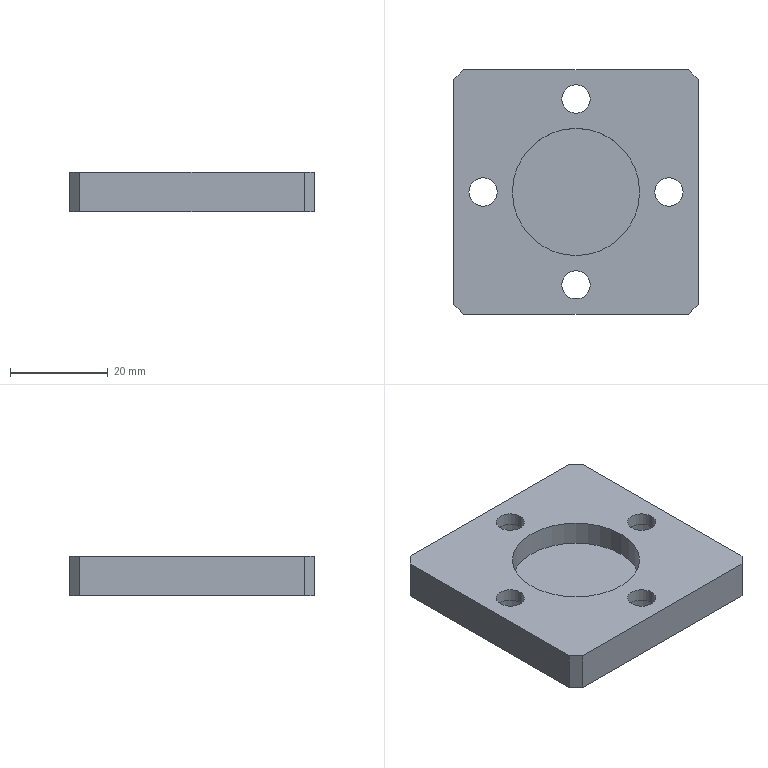Part | SolidWorks | features ICE 2, Chamfer 1, Extrusion 1, HoleWzd 1 | 1 solid | 33 faces | box 50 x 50 x 8 mm | volume 15310 mm3 | cylinder 18 | plane 15 | commonest cylinder face diameters 5.8 x8 10 x8 26 x2
STEP:
#1=CARTESIAN_POINT('',(5.,19.,1.4));
#2=VERTEX_POINT('',#1);
#3=CARTESIAN_POINT('',(-5.,19.,1.4));
#4=VERTEX_POINT('',#3);
#5=CARTESIAN_POINT('',(0.,19.,1.4));
#6=DIRECTION('',(0.,0.,-1.));
#7=DIRECTION('',(-1.,0.,0.));
#8=AXIS2_PLACEMENT_3D('',#5,#6,#7);
#9=CIRCLE('',#8,5.);
#10=EDGE_CURVE('',#2,#4,#9,.T.);
#11=ORIENTED_EDGE('',*,*,#10,.F.);
#12=CARTESIAN_POINT('',(5.,19.,-4.));
#13=VERTEX_POINT('',#12);
#14=CARTESIAN_POINT('',(5.,19.,-4.));
#15=DIRECTION('',(0.,0.,-1.));
#16=VECTOR('',#15,1000.);
#17=LINE('',#14,#16);
#18=EDGE_CURVE('',#2,#13,#17,.T.);
#19=ORIENTED_EDGE('',*,*,#18,.T.);
#20=CARTESIAN_POINT('',(-5.,19.,-4.));
#21=VERTEX_POINT('',#20);
#22=CARTESIAN_POINT('',(0.,19.,-4.));
#23=DIRECTION('',(0.,0.,-1.));
#24=DIRECTION('',(-1.,0.,0.));
#25=AXIS2_PLACEMENT_3D('',#22,#23,#24);
#26=CIRCLE('',#25,5.);
#27=EDGE_CURVE('',#13,#21,#26,.T.);
#28=ORIENTED_EDGE('',*,*,#27,.T.);
#29=CARTESIAN_POINT('',(-5.,19.,-4.));
#30=DIRECTION('',(0.,0.,-1.));
#31=VECTOR('',#30,1000.);
#32=LINE('',#29,#31);
#33=EDGE_CURVE('',#4,#21,#32,.T.);
#34=ORIENTED_EDGE('',*,*,#33,.F.);
#35=EDGE_LOOP('',(#11,#19,#28,#34));
#36=FACE_OUTER_BOUND('',#35,.T.);
#37=CARTESIAN_POINT('',(0.,19.,-4.));
#38=DIRECTION('',(0.,0.,-1.));
#39=DIRECTION('',(-1.,0.,0.));
#40=AXIS2_PLACEMENT_3D('',#37,#38,#39);
#41=CYLINDRICAL_SURFACE('',#40,5.);
#42=ADVANCED_FACE('',(#36),#41,.F.);
#43=CARTESIAN_POINT('',(2.9,19.,4.));
#44=VERTEX_POINT('',#43);
#45=CARTESIAN_POINT('',(-2.9,19.,4.));
#46=VERTEX_POINT('',#45);
#47=CARTESIAN_POINT('',(0.,19.,4.));
#48=DIRECTION('',(0.,0.,-1.));
#49=DIRECTION('',(-1.,0.,0.));
#50=AXIS2_PLACEMENT_3D('',#47,#48,#49);
#51=CIRCLE('',#50,2.9);
#52=EDGE_CURVE('',#44,#46,#51,.T.);
#53=ORIENTED_EDGE('',*,*,#52,.F.);
#54=CARTESIAN_POINT('',(2.9,19.,1.4));
#55=VERTEX_POINT('',#54);
#56=CARTESIAN_POINT('',(2.9,19.,-4.));
#57=DIRECTION('',(0.,0.,-1.));
#58=VECTOR('',#57,1000.);
#59=LINE('',#56,#58);
#60=EDGE_CURVE('',#44,#55,#59,.T.);
#61=ORIENTED_EDGE('',*,*,#60,.T.);
#62=CARTESIAN_POINT('',(-2.9,19.,1.4));
#63=VERTEX_POINT('',#62);
#64=CARTESIAN_POINT('',(0.,19.,1.4));
#65=DIRECTION('',(0.,0.,-1.));
#66=DIRECTION('',(-1.,0.,0.));
#67=AXIS2_PLACEMENT_3D('',#64,#65,#66);
#68=CIRCLE('',#67,2.9);
#69=EDGE_CURVE('',#55,#63,#68,.T.);
#70=ORIENTED_EDGE('',*,*,#69,.T.);
#71=CARTESIAN_POINT('',(-2.9,19.,-4.));
#72=DIRECTION('',(0.,0.,-1.));
#73=VECTOR('',#72,1000.);
#74=LINE('',#71,#73);
#75=EDGE_CURVE('',#46,#63,#74,.T.);
#76=ORIENTED_EDGE('',*,*,#75,.F.);
#77=EDGE_LOOP('',(#53,#61,#70,#76));
#78=FACE_OUTER_BOUND('',#77,.T.);
#79=CARTESIAN_POINT('',(0.,19.,-4.));
#80=DIRECTION('',(0.,0.,-1.));
#81=DIRECTION('',(-1.,0.,0.));
#82=AXIS2_PLACEMENT_3D('',#79,#80,#81);
#83=CYLINDRICAL_SURFACE('',#82,2.9);
#84=ADVANCED_FACE('',(#78),#83,.F.);
#85=CARTESIAN_POINT('',(24.,0.,1.4));
#86=VERTEX_POINT('',#85);
#87=CARTESIAN_POINT('',(14.,0.,1.4));
#88=VERTEX_POINT('',#87);
#89=CARTESIAN_POINT('',(19.,0.,1.4));
#90=DIRECTION('',(0.,0.,-1.));
#91=DIRECTION('',(-1.,0.,0.));
#92=AXIS2_PLACEMENT_3D('',#89,#90,#91);
#93=CIRCLE('',#92,5.);
#94=EDGE_CURVE('',#86,#88,#93,.T.);
#95=ORIENTED_EDGE('',*,*,#94,.F.);
#96=CARTESIAN_POINT('',(24.,0.,-4.));
#97=VERTEX_POINT('',#96);
#98=CARTESIAN_POINT('',(24.,0.,-4.));
#99=DIRECTION('',(0.,0.,-1.));
#100=VECTOR('',#99,1000.);
#101=LINE('',#98,#100);
#102=EDGE_CURVE('',#86,#97,#101,.T.);
#103=ORIENTED_EDGE('',*,*,#102,.T.);
#104=CARTESIAN_POINT('',(14.,0.,-4.));
#105=VERTEX_POINT('',#104);
#106=CARTESIAN_POINT('',(19.,0.,-4.));
#107=DIRECTION('',(0.,0.,-1.));
#108=DIRECTION('',(-1.,0.,0.));
#109=AXIS2_PLACEMENT_3D('',#106,#107,#108);
#110=CIRCLE('',#109,5.);
#111=EDGE_CURVE('',#97,#105,#110,.T.);
#112=ORIENTED_EDGE('',*,*,#111,.T.);
#113=CARTESIAN_POINT('',(14.,0.,-4.));
#114=DIRECTION('',(0.,0.,-1.));
#115=VECTOR('',#114,1000.);
#116=LINE('',#113,#115);
#117=EDGE_CURVE('',#88,#105,#116,.T.);
#118=ORIENTED_EDGE('',*,*,#117,.F.);
#119=EDGE_LOOP('',(#95,#103,#112,#118));
#120=FACE_OUTER_BOUND('',#119,.T.);
#121=CARTESIAN_POINT('',(19.,0.,-4.));
#122=DIRECTION('',(0.,0.,-1.));
#123=DIRECTION('',(-1.,0.,0.));
#124=AXIS2_PLACEMENT_3D('',#121,#122,#123);
#125=CYLINDRICAL_SURFACE('',#124,5.);
#126=ADVANCED_FACE('',(#120),#125,.F.);
#127=CARTESIAN_POINT('',(21.9,0.,4.));
#128=VERTEX_POINT('',#127);
#129=CARTESIAN_POINT('',(16.1,0.,4.));
#130=VERTEX_POINT('',#129);
#131=CARTESIAN_POINT('',(19.,0.,4.));
#132=DIRECTION('',(0.,0.,-1.));
#133=DIRECTION('',(-1.,0.,0.));
#134=AXIS2_PLACEMENT_3D('',#131,#132,#133);
#135=CIRCLE('',#134,2.9);
#136=EDGE_CURVE('',#128,#130,#135,.T.);
#137=ORIENTED_EDGE('',*,*,#136,.F.);
#138=CARTESIAN_POINT('',(21.9,0.,1.4));
#139=VERTEX_POINT('',#138);
#140=CARTESIAN_POINT('',(21.9,0.,-4.));
#141=DIRECTION('',(0.,0.,-1.));
#142=VECTOR('',#141,1000.);
#143=LINE('',#140,#142);
#144=EDGE_CURVE('',#128,#139,#143,.T.);
#145=ORIENTED_EDGE('',*,*,#144,.T.);
#146=CARTESIAN_POINT('',(16.1,0.,1.4));
#147=VERTEX_POINT('',#146);
#148=CARTESIAN_POINT('',(19.,0.,1.4));
#149=DIRECTION('',(0.,0.,-1.));
#150=DIRECTION('',(-1.,0.,0.));
#151=AXIS2_PLACEMENT_3D('',#148,#149,#150);
#152=CIRCLE('',#151,2.9);
#153=EDGE_CURVE('',#139,#147,#152,.T.);
#154=ORIENTED_EDGE('',*,*,#153,.T.);
#155=CARTESIAN_POINT('',(16.1,0.,-4.));
#156=DIRECTION('',(0.,0.,-1.));
#157=VECTOR('',#156,1000.);
#158=LINE('',#155,#157);
#159=EDGE_CURVE('',#130,#147,#158,.T.);
#160=ORIENTED_EDGE('',*,*,#159,.F.);
#161=EDGE_LOOP('',(#137,#145,#154,#160));
#162=FACE_OUTER_BOUND('',#161,.T.);
#163=CARTESIAN_POINT('',(19.,0.,-4.));
#164=DIRECTION('',(0.,0.,-1.));
#165=DIRECTION('',(-1.,0.,0.));
#166=AXIS2_PLACEMENT_3D('',#163,#164,#165);
#167=CYLINDRICAL_SURFACE('',#166,2.9);
#168=ADVANCED_FACE('',(#162),#167,.F.);
#169=CARTESIAN_POINT('',(5.,-19.,1.4));
#170=VERTEX_POINT('',#169);
#171=CARTESIAN_POINT('',(-5.,-19.,1.4));
#172=VERTEX_POINT('',#171);
#173=CARTESIAN_POINT('',(0.,-19.,1.4));
#174=DIRECTION('',(0.,0.,-1.));
#175=DIRECTION('',(-1.,0.,0.));
#176=AXIS2_PLACEMENT_3D('',#173,#174,#175);
#177=CIRCLE('',#176,5.);
#178=EDGE_CURVE('',#170,#172,#177,.T.);
#179=ORIENTED_EDGE('',*,*,#178,.F.);
#180=CARTESIAN_POINT('',(5.,-19.,-4.));
#181=VERTEX_POINT('',#180);
#182=CARTESIAN_POINT('',(5.,-19.,-4.));
#183=DIRECTION('',(0.,0.,-1.));
#184=VECTOR('',#183,1000.);
#185=LINE('',#182,#184);
#186=EDGE_CURVE('',#170,#181,#185,.T.);
#187=ORIENTED_EDGE('',*,*,#186,.T.);
#188=CARTESIAN_POINT('',(-5.,-19.,-4.));
#189=VERTEX_POINT('',#188);
#190=CARTESIAN_POINT('',(0.,-19.,-4.));
#191=DIRECTION('',(0.,0.,-1.));
#192=DIRECTION('',(-1.,0.,0.));
#193=AXIS2_PLACEMENT_3D('',#190,#191,#192);
#194=CIRCLE('',#193,5.);
#195=EDGE_CURVE('',#181,#189,#194,.T.);
#196=ORIENTED_EDGE('',*,*,#195,.T.);
#197=CARTESIAN_POINT('',(-5.,-19.,-4.));
#198=DIRECTION('',(0.,0.,-1.));
#199=VECTOR('',#198,1000.);
#200=LINE('',#197,#199);
#201=EDGE_CURVE('',#172,#189,#200,.T.);
#202=ORIENTED_EDGE('',*,*,#201,.F.);
#203=EDGE_LOOP('',(#179,#187,#196,#202));
#204=FACE_OUTER_BOUND('',#203,.T.);
#205=CARTESIAN_POINT('',(0.,-19.,-4.));
#206=DIRECTION('',(0.,0.,-1.));
#207=DIRECTION('',(-1.,0.,0.));
#208=AXIS2_PLACEMENT_3D('',#205,#206,#207);
#209=CYLINDRICAL_SURFACE('',#208,5.);
#210=ADVANCED_FACE('',(#204),#209,.F.);
#211=CARTESIAN_POINT('',(2.9,-19.,4.));
#212=VERTEX_POINT('',#211);
#213=CARTESIAN_POINT('',(-2.9,-19.,4.));
#214=VERTEX_POINT('',#213);
#215=CARTESIAN_POINT('',(0.,-19.,4.));
#216=DIRECTION('',(0.,0.,-1.));
#217=DIRECTION('',(-1.,0.,0.));
#218=AXIS2_PLACEMENT_3D('',#215,#216,#217);
#219=CIRCLE('',#218,2.9);
#220=EDGE_CURVE('',#212,#214,#219,.T.);
#221=ORIENTED_EDGE('',*,*,#220,.F.);
#222=CARTESIAN_POINT('',(2.9,-19.,1.4));
#223=VERTEX_POINT('',#222);
#224=CARTESIAN_POINT('',(2.9,-19.,-4.));
#225=DIRECTION('',(0.,0.,-1.));
#226=VECTOR('',#225,1000.);
#227=LINE('',#224,#226);
#228=EDGE_CURVE('',#212,#223,#227,.T.);
#229=ORIENTED_EDGE('',*,*,#228,.T.);
#230=CARTESIAN_POINT('',(-2.9,-19.,1.4));
#231=VERTEX_POINT('',#230);
#232=CARTESIAN_POINT('',(0.,-19.,1.4));
#233=DIRECTION('',(0.,0.,-1.));
#234=DIRECTION('',(-1.,0.,0.));
#235=AXIS2_PLACEMENT_3D('',#232,#233,#234);
#236=CIRCLE('',#235,2.9);
#237=EDGE_CURVE('',#223,#231,#236,.T.);
#238=ORIENTED_EDGE('',*,*,#237,.T.);
#239=CARTESIAN_POINT('',(-2.9,-19.,-4.));
#240=DIRECTION('',(0.,0.,-1.));
#241=VECTOR('',#240,1000.);
#242=LINE('',#239,#241);
#243=EDGE_CURVE('',#214,#231,#242,.T.);
#244=ORIENTED_EDGE('',*,*,#243,.F.);
#245=EDGE_LOOP('',(#221,#229,#238,#244));
#246=FACE_OUTER_BOUND('',#245,.T.);
#247=CARTESIAN_POINT('',(0.,-19.,-4.));
#248=DIRECTION('',(0.,0.,-1.));
#249=DIRECTION('',(-1.,0.,0.));
#250=AXIS2_PLACEMENT_3D('',#247,#248,#249);
#251=CYLINDRICAL_SURFACE('',#250,2.9);
#252=ADVANCED_FACE('',(#246),#251,.F.);
#253=CARTESIAN_POINT('',(-14.,0.,1.4));
#254=VERTEX_POINT('',#253);
#255=CARTESIAN_POINT('',(-24.,0.,1.4));
#256=VERTEX_POINT('',#255);
#257=CARTESIAN_POINT('',(-19.,0.,1.4));
#258=DIRECTION('',(0.,0.,-1.));
#259=DIRECTION('',(-1.,0.,0.));
#260=AXIS2_PLACEMENT_3D('',#257,#258,#259);
#261=CIRCLE('',#260,5.);
#262=EDGE_CURVE('',#254,#256,#261,.T.);
#263=ORIENTED_EDGE('',*,*,#262,.F.);
#264=CARTESIAN_POINT('',(-14.,0.,-4.));
#265=VERTEX_POINT('',#264);
#266=CARTESIAN_POINT('',(-14.,0.,-4.));
#267=DIRECTION('',(0.,0.,-1.));
#268=VECTOR('',#267,1000.);
#269=LINE('',#266,#268);
#270=EDGE_CURVE('',#254,#265,#269,.T.);
#271=ORIENTED_EDGE('',*,*,#270,.T.);
#272=CARTESIAN_POINT('',(-24.,0.,-4.));
#273=VERTEX_POINT('',#272);
#274=CARTESIAN_POINT('',(-19.,0.,-4.));
#275=DIRECTION('',(0.,0.,-1.));
#276=DIRECTION('',(-1.,0.,0.));
#277=AXIS2_PLACEMENT_3D('',#274,#275,#276);
#278=CIRCLE('',#277,5.);
#279=EDGE_CURVE('',#265,#273,#278,.T.);
#280=ORIENTED_EDGE('',*,*,#279,.T.);
#281=CARTESIAN_POINT('',(-24.,0.,-4.));
#282=DIRECTION('',(0.,0.,-1.));
#283=VECTOR('',#282,1000.);
#284=LINE('',#281,#283);
#285=EDGE_CURVE('',#256,#273,#284,.T.);
#286=ORIENTED_EDGE('',*,*,#285,.F.);
#287=EDGE_LOOP('',(#263,#271,#280,#286));
#288=FACE_OUTER_BOUND('',#287,.T.);
#289=CARTESIAN_POINT('',(-19.,0.,-4.));
#290=DIRECTION('',(0.,0.,-1.));
#291=DIRECTION('',(-1.,0.,0.));
#292=AXIS2_PLACEMENT_3D('',#289,#290,#291);
#293=CYLINDRICAL_SURFACE('',#292,5.);
#294=ADVANCED_FACE('',(#288),#293,.F.);
#295=CARTESIAN_POINT('',(-16.1,0.,4.));
#296=VERTEX_POINT('',#295);
#297=CARTESIAN_POINT('',(-21.9,0.,4.));
#298=VERTEX_POINT('',#297);
#299=CARTESIAN_POINT('',(-19.,0.,4.));
#300=DIRECTION('',(0.,0.,-1.));
#301=DIRECTION('',(-1.,0.,0.));
#302=AXIS2_PLACEMENT_3D('',#299,#300,#301);
#303=CIRCLE('',#302,2.9);
#304=EDGE_CURVE('',#296,#298,#303,.T.);
#305=ORIENTED_EDGE('',*,*,#304,.F.);
#306=CARTESIAN_POINT('',(-16.1,0.,1.4));
#307=VERTEX_POINT('',#306);
#308=CARTESIAN_POINT('',(-16.1,0.,-4.));
#309=DIRECTION('',(0.,0.,-1.));
#310=VECTOR('',#309,1000.);
#311=LINE('',#308,#310);
#312=EDGE_CURVE('',#296,#307,#311,.T.);
#313=ORIENTED_EDGE('',*,*,#312,.T.);
#314=CARTESIAN_POINT('',(-21.9,0.,1.4));
#315=VERTEX_POINT('',#314);
#316=CARTESIAN_POINT('',(-19.,0.,1.4));
#317=DIRECTION('',(0.,0.,-1.));
#318=DIRECTION('',(-1.,0.,0.));
#319=AXIS2_PLACEMENT_3D('',#316,#317,#318);
#320=CIRCLE('',#319,2.9);
#321=EDGE_CURVE('',#307,#315,#320,.T.);
#322=ORIENTED_EDGE('',*,*,#321,.T.);
#323=CARTESIAN_POINT('',(-21.9,0.,-4.));
#324=DIRECTION('',(0.,0.,-1.));
#325=VECTOR('',#324,1000.);
#326=LINE('',#323,#325);
#327=EDGE_CURVE('',#298,#315,#326,.T.);
#328=ORIENTED_EDGE('',*,*,#327,.F.);
#329=EDGE_LOOP('',(#305,#313,#322,#328));
#330=FACE_OUTER_BOUND('',#329,.T.);
#331=CARTESIAN_POINT('',(-19.,0.,-4.));
#332=DIRECTION('',(0.,0.,-1.));
#333=DIRECTION('',(-1.,0.,0.));
#334=AXIS2_PLACEMENT_3D('',#331,#332,#333);
#335=CYLINDRICAL_SURFACE('',#334,2.9);
#336=ADVANCED_FACE('',(#330),#335,.F.);
#337=CARTESIAN_POINT('',(-13.,0.,-1.));
#338=VERTEX_POINT('',#337);
#339=CARTESIAN_POINT('',(13.,0.,-1.));
#340=VERTEX_POINT('',#339);
#341=CARTESIAN_POINT('',(0.,0.,-1.));
#342=DIRECTION('',(0.,0.,1.));
#343=DIRECTION('',(1.,0.,0.));
#344=AXIS2_PLACEMENT_3D('',#341,#342,#343);
#345=CIRCLE('',#344,13.);
#346=EDGE_CURVE('',#338,#340,#345,.T.);
#347=ORIENTED_EDGE('',*,*,#346,.F.);
#348=CARTESIAN_POINT('',(-13.,0.,4.));
#349=VERTEX_POINT('',#348);
#350=CARTESIAN_POINT('',(-13.,0.,-1.));
#351=DIRECTION('',(0.,0.,1.));
#352=VECTOR('',#351,1000.);
#353=LINE('',#350,#352);
#354=EDGE_CURVE('',#338,#349,#353,.T.);
#355=ORIENTED_EDGE('',*,*,#354,.T.);
#356=CARTESIAN_POINT('',(13.,0.,4.));
#357=VERTEX_POINT('',#356);
#358=CARTESIAN_POINT('',(0.,0.,4.));
#359=DIRECTION('',(0.,0.,1.));
#360=DIRECTION('',(1.,0.,0.));
#361=AXIS2_PLACEMENT_3D('',#358,#359,#360);
#362=CIRCLE('',#361,13.);
#363=EDGE_CURVE('',#349,#357,#362,.T.);
#364=ORIENTED_EDGE('',*,*,#363,.T.);
#365=CARTESIAN_POINT('',(13.,0.,-1.));
#366=DIRECTION('',(0.,0.,1.));
#367=VECTOR('',#366,1000.);
#368=LINE('',#365,#367);
#369=EDGE_CURVE('',#340,#357,#368,.T.);
#370=ORIENTED_EDGE('',*,*,#369,.F.);
#371=EDGE_LOOP('',(#347,#355,#364,#370));
#372=FACE_OUTER_BOUND('',#371,.T.);
#373=CARTESIAN_POINT('',(0.,0.,-1.));
#374=DIRECTION('',(0.,0.,1.));
#375=DIRECTION('',(1.,0.,0.));
#376=AXIS2_PLACEMENT_3D('',#373,#374,#375);
#377=CYLINDRICAL_SURFACE('',#376,13.);
#378=ADVANCED_FACE('',(#372),#377,.F.);
#379=CARTESIAN_POINT('',(25.,-23.,4.));
#380=VERTEX_POINT('',#379);
#381=CARTESIAN_POINT('',(25.,23.,4.));
#382=VERTEX_POINT('',#381);
#383=CARTESIAN_POINT('',(25.,-25.,4.));
#384=DIRECTION('',(0.,1.,0.));
#385=VECTOR('',#384,1000.);
#386=LINE('',#383,#385);
#387=EDGE_CURVE('',#380,#382,#386,.T.);
#388=ORIENTED_EDGE('',*,*,#387,.F.);
#389=CARTESIAN_POINT('',(25.,-23.,-4.));
#390=VERTEX_POINT('',#389);
#391=CARTESIAN_POINT('',(25.,-23.,4.));
#392=DIRECTION('',(0.,0.,-1.));
#393=VECTOR('',#392,1000.);
#394=LINE('',#391,#393);
#395=EDGE_CURVE('',#380,#390,#394,.T.);
#396=ORIENTED_EDGE('',*,*,#395,.T.);
#397=CARTESIAN_POINT('',(25.,23.,-4.));
#398=VERTEX_POINT('',#397);
#399=CARTESIAN_POINT('',(25.,-25.,-4.));
#400=DIRECTION('',(0.,1.,0.));
#401=VECTOR('',#400,1000.);
#402=LINE('',#399,#401);
#403=EDGE_CURVE('',#390,#398,#402,.T.);
#404=ORIENTED_EDGE('',*,*,#403,.T.);
#405=CARTESIAN_POINT('',(25.,23.,4.));
#406=DIRECTION('',(0.,0.,1.));
#407=VECTOR('',#406,1000.);
#408=LINE('',#405,#407);
#409=EDGE_CURVE('',#398,#382,#408,.T.);
#410=ORIENTED_EDGE('',*,*,#409,.T.);
#411=EDGE_LOOP('',(#388,#396,#404,#410));
#412=FACE_OUTER_BOUND('',#411,.T.);
#413=CARTESIAN_POINT('',(25.,-25.,4.));
#414=DIRECTION('',(-1.,0.,0.));
#415=DIRECTION('',(0.,0.,1.));
#416=AXIS2_PLACEMENT_3D('',#413,#414,#415);
#417=PLANE('',#416);
#418=ADVANCED_FACE('',(#412),#417,.F.);
#419=CARTESIAN_POINT('',(23.,25.,4.));
#420=VERTEX_POINT('',#419);
#421=CARTESIAN_POINT('',(-23.,25.,4.));
#422=VERTEX_POINT('',#421);
#423=CARTESIAN_POINT('',(-25.,25.,4.));
#424=DIRECTION('',(-1.,0.,0.));
#425=VECTOR('',#424,1000.);
#426=LINE('',#423,#425);
#427=EDGE_CURVE('',#420,#422,#426,.T.);
#428=ORIENTED_EDGE('',*,*,#427,.F.);
#429=CARTESIAN_POINT('',(23.,25.,-4.));
#430=VERTEX_POINT('',#429);
#431=CARTESIAN_POINT('',(23.,25.,4.));
#432=DIRECTION('',(0.,0.,-1.));
#433=VECTOR('',#432,1000.);
#434=LINE('',#431,#433);
#435=EDGE_CURVE('',#420,#430,#434,.T.);
#436=ORIENTED_EDGE('',*,*,#435,.T.);
#437=CARTESIAN_POINT('',(-23.,25.,-4.));
#438=VERTEX_POINT('',#437);
#439=CARTESIAN_POINT('',(-25.,25.,-4.));
#440=DIRECTION('',(-1.,0.,0.));
#441=VECTOR('',#440,1000.);
#442=LINE('',#439,#441);
#443=EDGE_CURVE('',#430,#438,#442,.T.);
#444=ORIENTED_EDGE('',*,*,#443,.T.);
#445=CARTESIAN_POINT('',(-23.,25.,4.));
#446=DIRECTION('',(0.,0.,1.));
#447=VECTOR('',#446,1000.);
#448=LINE('',#445,#447);
#449=EDGE_CURVE('',#438,#422,#448,.T.);
#450=ORIENTED_EDGE('',*,*,#449,.T.);
#451=EDGE_LOOP('',(#428,#436,#444,#450));
#452=FACE_OUTER_BOUND('',#451,.T.);
#453=CARTESIAN_POINT('',(-25.,25.,4.));
#454=DIRECTION('',(0.,-1.,0.));
#455=DIRECTION('',(0.,0.,-1.));
#456=AXIS2_PLACEMENT_3D('',#453,#454,#455);
#457=PLANE('',#456);
#458=ADVANCED_FACE('',(#452),#457,.F.);
#459=CARTESIAN_POINT('',(-25.,23.,-4.));
#460=VERTEX_POINT('',#459);
#461=CARTESIAN_POINT('',(-25.,-23.,-4.));
#462=VERTEX_POINT('',#461);
#463=CARTESIAN_POINT('',(-25.,-25.,-4.));
#464=DIRECTION('',(0.,-1.,0.));
#465=VECTOR('',#464,1000.);
#466=LINE('',#463,#465);
#467=EDGE_CURVE('',#460,#462,#466,.T.);
#468=ORIENTED_EDGE('',*,*,#467,.T.);
#469=CARTESIAN_POINT('',(-25.,-23.,4.));
#470=VERTEX_POINT('',#469);
#471=CARTESIAN_POINT('',(-25.,-23.,4.));
#472=DIRECTION('',(0.,0.,1.));
#473=VECTOR('',#472,1000.);
#474=LINE('',#471,#473);
#475=EDGE_CURVE('',#462,#470,#474,.T.);
#476=ORIENTED_EDGE('',*,*,#475,.T.);
#477=CARTESIAN_POINT('',(-25.,23.,4.));
#478=VERTEX_POINT('',#477);
#479=CARTESIAN_POINT('',(-25.,-25.,4.));
#480=DIRECTION('',(0.,-1.,0.));
#481=VECTOR('',#480,1000.);
#482=LINE('',#479,#481);
#483=EDGE_CURVE('',#478,#470,#482,.T.);
#484=ORIENTED_EDGE('',*,*,#483,.F.);
#485=CARTESIAN_POINT('',(-25.,23.,4.));
#486=DIRECTION('',(0.,0.,-1.));
#487=VECTOR('',#486,1000.);
#488=LINE('',#485,#487);
#489=EDGE_CURVE('',#478,#460,#488,.T.);
#490=ORIENTED_EDGE('',*,*,#489,.T.);
#491=EDGE_LOOP('',(#468,#476,#484,#490));
#492=FACE_OUTER_BOUND('',#491,.T.);
#493=CARTESIAN_POINT('',(-25.,-25.,4.));
#494=DIRECTION('',(1.,0.,0.));
#495=DIRECTION('',(0.,0.,-1.));
#496=AXIS2_PLACEMENT_3D('',#493,#494,#495);
#497=PLANE('',#496);
#498=ADVANCED_FACE('',(#492),#497,.F.);
#499=CARTESIAN_POINT('',(-23.,-25.,4.));
#500=VERTEX_POINT('',#499);
#501=CARTESIAN_POINT('',(23.,-25.,4.));
#502=VERTEX_POINT('',#501);
#503=CARTESIAN_POINT('',(-25.,-25.,4.));
#504=DIRECTION('',(1.,0.,0.));
#505=VECTOR('',#504,1000.);
#506=LINE('',#503,#505);
#507=EDGE_CURVE('',#500,#502,#506,.T.);
#508=ORIENTED_EDGE('',*,*,#507,.F.);
#509=CARTESIAN_POINT('',(-23.,-25.,-4.));
#510=VERTEX_POINT('',#509);
#511=CARTESIAN_POINT('',(-23.,-25.,4.));
#512=DIRECTION('',(0.,0.,-1.));
#513=VECTOR('',#512,1000.);
#514=LINE('',#511,#513);
#515=EDGE_CURVE('',#500,#510,#514,.T.);
#516=ORIENTED_EDGE('',*,*,#515,.T.);
#517=CARTESIAN_POINT('',(23.,-25.,-4.));
#518=VERTEX_POINT('',#517);
#519=CARTESIAN_POINT('',(-25.,-25.,-4.));
#520=DIRECTION('',(1.,0.,0.));
#521=VECTOR('',#520,1000.);
#522=LINE('',#519,#521);
#523=EDGE_CURVE('',#510,#518,#522,.T.);
#524=ORIENTED_EDGE('',*,*,#523,.T.);
#525=CARTESIAN_POINT('',(23.,-25.,4.));
#526=DIRECTION('',(0.,0.,1.));
#527=VECTOR('',#526,1000.);
#528=LINE('',#525,#527);
#529=EDGE_CURVE('',#518,#502,#528,.T.);
#530=ORIENTED_EDGE('',*,*,#529,.T.);
#531=EDGE_LOOP('',(#508,#516,#524,#530));
#532=FACE_OUTER_BOUND('',#531,.T.);
#533=CARTESIAN_POINT('',(-25.,-25.,4.));
#534=DIRECTION('',(0.,1.,0.));
#535=DIRECTION('',(0.,0.,1.));
#536=AXIS2_PLACEMENT_3D('',#533,#534,#535);
#537=PLANE('',#536);
#538=ADVANCED_FACE('',(#532),#537,.F.);
#539=CARTESIAN_POINT('',(0.,19.,4.));
#540=DIRECTION('',(0.,0.,-1.));
#541=DIRECTION('',(-1.,0.,0.));
#542=AXIS2_PLACEMENT_3D('',#539,#540,#541);
#543=CIRCLE('',#542,2.9);
#544=EDGE_CURVE('',#46,#44,#543,.T.);
#545=ORIENTED_EDGE('',*,*,#544,.T.);
#546=ORIENTED_EDGE('',*,*,#52,.T.);
#547=EDGE_LOOP('',(#545,#546));
#548=FACE_BOUND('',#547,.T.);
#549=CARTESIAN_POINT('',(19.,0.,4.));
#550=DIRECTION('',(0.,0.,-1.));
#551=DIRECTION('',(-1.,0.,0.));
#552=AXIS2_PLACEMENT_3D('',#549,#550,#551);
#553=CIRCLE('',#552,2.9);
#554=EDGE_CURVE('',#130,#128,#553,.T.);
#555=ORIENTED_EDGE('',*,*,#554,.T.);
#556=ORIENTED_EDGE('',*,*,#136,.T.);
#557=EDGE_LOOP('',(#555,#556));
#558=FACE_BOUND('',#557,.T.);
#559=CARTESIAN_POINT('',(0.,-19.,4.));
#560=DIRECTION('',(0.,0.,-1.));
#561=DIRECTION('',(-1.,0.,0.));
#562=AXIS2_PLACEMENT_3D('',#559,#560,#561);
#563=CIRCLE('',#562,2.9);
#564=EDGE_CURVE('',#214,#212,#563,.T.);
#565=ORIENTED_EDGE('',*,*,#564,.T.);
#566=ORIENTED_EDGE('',*,*,#220,.T.);
#567=EDGE_LOOP('',(#565,#566));
#568=FACE_BOUND('',#567,.T.);
#569=CARTESIAN_POINT('',(-19.,0.,4.));
#570=DIRECTION('',(0.,0.,-1.));
#571=DIRECTION('',(-1.,0.,0.));
#572=AXIS2_PLACEMENT_3D('',#569,#570,#571);
#573=CIRCLE('',#572,2.9);
#574=EDGE_CURVE('',#298,#296,#573,.T.);
#575=ORIENTED_EDGE('',*,*,#574,.T.);
#576=ORIENTED_EDGE('',*,*,#304,.T.);
#577=EDGE_LOOP('',(#575,#576));
#578=FACE_BOUND('',#577,.T.);
#579=CARTESIAN_POINT('',(0.,0.,4.));
#580=DIRECTION('',(0.,0.,1.));
#581=DIRECTION('',(1.,0.,0.));
#582=AXIS2_PLACEMENT_3D('',#579,#580,#581);
#583=CIRCLE('',#582,13.);
#584=EDGE_CURVE('',#357,#349,#583,.T.);
#585=ORIENTED_EDGE('',*,*,#584,.F.);
#586=ORIENTED_EDGE('',*,*,#363,.F.);
#587=EDGE_LOOP('',(#585,#586));
#588=FACE_BOUND('',#587,.T.);
#589=ORIENTED_EDGE('',*,*,#483,.T.);
#590=CARTESIAN_POINT('',(-23.,-25.,4.));
#591=DIRECTION('',(0.7071,-0.7071,0.));
#592=VECTOR('',#591,1000.);
#593=LINE('',#590,#592);
#594=EDGE_CURVE('',#470,#500,#593,.T.);
#595=ORIENTED_EDGE('',*,*,#594,.T.);
#596=ORIENTED_EDGE('',*,*,#507,.T.);
#597=CARTESIAN_POINT('',(25.,-23.,4.));
#598=DIRECTION('',(0.7071,0.7071,0.));
#599=VECTOR('',#598,1000.);
#600=LINE('',#597,#599);
#601=EDGE_CURVE('',#502,#380,#600,.T.);
#602=ORIENTED_EDGE('',*,*,#601,.T.);
#603=ORIENTED_EDGE('',*,*,#387,.T.);
#604=CARTESIAN_POINT('',(23.,25.,4.));
#605=DIRECTION('',(-0.7071,0.7071,0.));
#606=VECTOR('',#605,1000.);
#607=LINE('',#604,#606);
#608=EDGE_CURVE('',#382,#420,#607,.T.);
#609=ORIENTED_EDGE('',*,*,#608,.T.);
#610=ORIENTED_EDGE('',*,*,#427,.T.);
#611=CARTESIAN_POINT('',(-25.,23.,4.));
#612=DIRECTION('',(-0.7071,-0.7071,0.));
#613=VECTOR('',#612,1000.);
#614=LINE('',#611,#613);
#615=EDGE_CURVE('',#422,#478,#614,.T.);
#616=ORIENTED_EDGE('',*,*,#615,.T.);
#617=EDGE_LOOP('',(#589,#595,#596,#602,#603,#609,#610,#616));
#618=FACE_OUTER_BOUND('',#617,.T.);
#619=CARTESIAN_POINT('',(0.,0.,4.));
#620=DIRECTION('',(0.,0.,-1.));
#621=DIRECTION('',(-1.,0.,0.));
#622=AXIS2_PLACEMENT_3D('',#619,#620,#621);
#623=PLANE('',#622);
#624=ADVANCED_FACE('',(#548,#558,#568,#578,#588,#618),#623,.F.);
#625=CARTESIAN_POINT('',(0.,19.,-4.));
#626=DIRECTION('',(0.,0.,-1.));
#627=DIRECTION('',(-1.,0.,0.));
#628=AXIS2_PLACEMENT_3D('',#625,#626,#627);
#629=CIRCLE('',#628,5.);
#630=EDGE_CURVE('',#21,#13,#629,.T.);
#631=ORIENTED_EDGE('',*,*,#630,.F.);
#632=ORIENTED_EDGE('',*,*,#27,.F.);
#633=EDGE_LOOP('',(#631,#632));
#634=FACE_BOUND('',#633,.T.);
#635=CARTESIAN_POINT('',(19.,0.,-4.));
#636=DIRECTION('',(0.,0.,-1.));
#637=DIRECTION('',(-1.,0.,0.));
#638=AXIS2_PLACEMENT_3D('',#635,#636,#637);
#639=CIRCLE('',#638,5.);
#640=EDGE_CURVE('',#105,#97,#639,.T.);
#641=ORIENTED_EDGE('',*,*,#640,.F.);
#642=ORIENTED_EDGE('',*,*,#111,.F.);
#643=EDGE_LOOP('',(#641,#642));
#644=FACE_BOUND('',#643,.T.);
#645=CARTESIAN_POINT('',(0.,-19.,-4.));
#646=DIRECTION('',(0.,0.,-1.));
#647=DIRECTION('',(-1.,0.,0.));
#648=AXIS2_PLACEMENT_3D('',#645,#646,#647);
#649=CIRCLE('',#648,5.);
#650=EDGE_CURVE('',#189,#181,#649,.T.);
#651=ORIENTED_EDGE('',*,*,#650,.F.);
#652=ORIENTED_EDGE('',*,*,#195,.F.);
#653=EDGE_LOOP('',(#651,#652));
#654=FACE_BOUND('',#653,.T.);
#655=CARTESIAN_POINT('',(-19.,0.,-4.));
#656=DIRECTION('',(0.,0.,-1.));
#657=DIRECTION('',(-1.,0.,0.));
#658=AXIS2_PLACEMENT_3D('',#655,#656,#657);
#659=CIRCLE('',#658,5.);
#660=EDGE_CURVE('',#273,#265,#659,.T.);
#661=ORIENTED_EDGE('',*,*,#660,.F.);
#662=ORIENTED_EDGE('',*,*,#279,.F.);
#663=EDGE_LOOP('',(#661,#662));
#664=FACE_BOUND('',#663,.T.);
#665=ORIENTED_EDGE('',*,*,#523,.F.);
#666=CARTESIAN_POINT('',(-24.,-24.,-4.));
#667=DIRECTION('',(-0.7071,0.7071,0.));
#668=VECTOR('',#667,1000.);
#669=LINE('',#666,#668);
#670=EDGE_CURVE('',#510,#462,#669,.T.);
#671=ORIENTED_EDGE('',*,*,#670,.T.);
#672=ORIENTED_EDGE('',*,*,#467,.F.);
#673=CARTESIAN_POINT('',(-24.,24.,-4.));
#674=DIRECTION('',(0.7071,0.7071,0.));
#675=VECTOR('',#674,1000.);
#676=LINE('',#673,#675);
#677=EDGE_CURVE('',#460,#438,#676,.T.);
#678=ORIENTED_EDGE('',*,*,#677,.T.);
#679=ORIENTED_EDGE('',*,*,#443,.F.);
#680=CARTESIAN_POINT('',(24.,24.,-4.));
#681=DIRECTION('',(0.7071,-0.7071,0.));
#682=VECTOR('',#681,1000.);
#683=LINE('',#680,#682);
#684=EDGE_CURVE('',#430,#398,#683,.T.);
#685=ORIENTED_EDGE('',*,*,#684,.T.);
#686=ORIENTED_EDGE('',*,*,#403,.F.);
#687=CARTESIAN_POINT('',(24.,-24.,-4.));
#688=DIRECTION('',(-0.7071,-0.7071,0.));
#689=VECTOR('',#688,1000.);
#690=LINE('',#687,#689);
#691=EDGE_CURVE('',#390,#518,#690,.T.);
#692=ORIENTED_EDGE('',*,*,#691,.T.);
#693=EDGE_LOOP('',(#665,#671,#672,#678,#679,#685,#686,#692));
#694=FACE_OUTER_BOUND('',#693,.T.);
#695=CARTESIAN_POINT('',(0.,0.,-4.));
#696=DIRECTION('',(0.,0.,-1.));
#697=DIRECTION('',(-1.,0.,0.));
#698=AXIS2_PLACEMENT_3D('',#695,#696,#697);
#699=PLANE('',#698);
#700=ADVANCED_FACE('',(#634,#644,#654,#664,#694),#699,.T.);
#701=ORIENTED_EDGE('',*,*,#354,.F.);
#702=CARTESIAN_POINT('',(0.,0.,-1.));
#703=DIRECTION('',(0.,0.,1.));
#704=DIRECTION('',(1.,0.,0.));
#705=AXIS2_PLACEMENT_3D('',#702,#703,#704);
#706=CIRCLE('',#705,13.);
#707=EDGE_CURVE('',#340,#338,#706,.T.);
#708=ORIENTED_EDGE('',*,*,#707,.F.);
#709=ORIENTED_EDGE('',*,*,#369,.T.);
#710=ORIENTED_EDGE('',*,*,#584,.T.);
#711=EDGE_LOOP('',(#701,#708,#709,#710));
#712=FACE_OUTER_BOUND('',#711,.T.);
#713=CARTESIAN_POINT('',(0.,0.,-1.));
#714=DIRECTION('',(0.,0.,1.));
#715=DIRECTION('',(1.,0.,0.));
#716=AXIS2_PLACEMENT_3D('',#713,#714,#715);
#717=CYLINDRICAL_SURFACE('',#716,13.);
#718=ADVANCED_FACE('',(#712),#717,.F.);
#719=ORIENTED_EDGE('',*,*,#707,.T.);
#720=ORIENTED_EDGE('',*,*,#346,.T.);
#721=EDGE_LOOP('',(#719,#720));
#722=FACE_OUTER_BOUND('',#721,.T.);
#723=CARTESIAN_POINT('',(0.,0.,-1.));
#724=DIRECTION('',(0.,0.,1.));
#725=DIRECTION('',(1.,0.,0.));
#726=AXIS2_PLACEMENT_3D('',#723,#724,#725);
#727=PLANE('',#726);
#728=ADVANCED_FACE('',(#722),#727,.T.);
#729=ORIENTED_EDGE('',*,*,#312,.F.);
#730=ORIENTED_EDGE('',*,*,#574,.F.);
#731=ORIENTED_EDGE('',*,*,#327,.T.);
#732=CARTESIAN_POINT('',(-19.,0.,1.4));
#733=DIRECTION('',(0.,0.,-1.));
#734=DIRECTION('',(-1.,0.,0.));
#735=AXIS2_PLACEMENT_3D('',#732,#733,#734);
#736=CIRCLE('',#735,2.9);
#737=EDGE_CURVE('',#315,#307,#736,.T.);
#738=ORIENTED_EDGE('',*,*,#737,.T.);
#739=EDGE_LOOP('',(#729,#730,#731,#738));
#740=FACE_OUTER_BOUND('',#739,.T.);
#741=CARTESIAN_POINT('',(-19.,0.,-4.));
#742=DIRECTION('',(0.,0.,-1.));
#743=DIRECTION('',(-1.,0.,0.));
#744=AXIS2_PLACEMENT_3D('',#741,#742,#743);
#745=CYLINDRICAL_SURFACE('',#744,2.9);
#746=ADVANCED_FACE('',(#740),#745,.F.);
#747=ORIENTED_EDGE('',*,*,#737,.F.);
#748=ORIENTED_EDGE('',*,*,#321,.F.);
#749=EDGE_LOOP('',(#747,#748));
#750=FACE_BOUND('',#749,.T.);
#751=CARTESIAN_POINT('',(-19.,0.,1.4));
#752=DIRECTION('',(0.,0.,-1.));
#753=DIRECTION('',(-1.,0.,0.));
#754=AXIS2_PLACEMENT_3D('',#751,#752,#753);
#755=CIRCLE('',#754,5.);
#756=EDGE_CURVE('',#256,#254,#755,.T.);
#757=ORIENTED_EDGE('',*,*,#756,.T.);
#758=ORIENTED_EDGE('',*,*,#262,.T.);
#759=EDGE_LOOP('',(#757,#758));
#760=FACE_OUTER_BOUND('',#759,.T.);
#761=CARTESIAN_POINT('',(-16.1,0.,1.4));
#762=DIRECTION('',(0.,0.,1.));
#763=DIRECTION('',(1.,0.,0.));
#764=AXIS2_PLACEMENT_3D('',#761,#762,#763);
#765=PLANE('',#764);
#766=ADVANCED_FACE('',(#750,#760),#765,.F.);
#767=ORIENTED_EDGE('',*,*,#270,.F.);
#768=ORIENTED_EDGE('',*,*,#756,.F.);
#769=ORIENTED_EDGE('',*,*,#285,.T.);
#770=ORIENTED_EDGE('',*,*,#660,.T.);
#771=EDGE_LOOP('',(#767,#768,#769,#770));
#772=FACE_OUTER_BOUND('',#771,.T.);
#773=CARTESIAN_POINT('',(-19.,0.,-4.));
#774=DIRECTION('',(0.,0.,-1.));
#775=DIRECTION('',(-1.,0.,0.));
#776=AXIS2_PLACEMENT_3D('',#773,#774,#775);
#777=CYLINDRICAL_SURFACE('',#776,5.);
#778=ADVANCED_FACE('',(#772),#777,.F.);
#779=ORIENTED_EDGE('',*,*,#228,.F.);
#780=ORIENTED_EDGE('',*,*,#564,.F.);
#781=ORIENTED_EDGE('',*,*,#243,.T.);
#782=CARTESIAN_POINT('',(0.,-19.,1.4));
#783=DIRECTION('',(0.,0.,-1.));
#784=DIRECTION('',(-1.,0.,0.));
#785=AXIS2_PLACEMENT_3D('',#782,#783,#784);
#786=CIRCLE('',#785,2.9);
#787=EDGE_CURVE('',#231,#223,#786,.T.);
#788=ORIENTED_EDGE('',*,*,#787,.T.);
#789=EDGE_LOOP('',(#779,#780,#781,#788));
#790=FACE_OUTER_BOUND('',#789,.T.);
#791=CARTESIAN_POINT('',(0.,-19.,-4.));
#792=DIRECTION('',(0.,0.,-1.));
#793=DIRECTION('',(-1.,0.,0.));
#794=AXIS2_PLACEMENT_3D('',#791,#792,#793);
#795=CYLINDRICAL_SURFACE('',#794,2.9);
#796=ADVANCED_FACE('',(#790),#795,.F.);
#797=ORIENTED_EDGE('',*,*,#787,.F.);
#798=ORIENTED_EDGE('',*,*,#237,.F.);
#799=EDGE_LOOP('',(#797,#798));
#800=FACE_BOUND('',#799,.T.);
#801=CARTESIAN_POINT('',(0.,-19.,1.4));
#802=DIRECTION('',(0.,0.,-1.));
#803=DIRECTION('',(-1.,0.,0.));
#804=AXIS2_PLACEMENT_3D('',#801,#802,#803);
#805=CIRCLE('',#804,5.);
#806=EDGE_CURVE('',#172,#170,#805,.T.);
#807=ORIENTED_EDGE('',*,*,#806,.T.);
#808=ORIENTED_EDGE('',*,*,#178,.T.);
#809=EDGE_LOOP('',(#807,#808));
#810=FACE_OUTER_BOUND('',#809,.T.);
#811=CARTESIAN_POINT('',(2.9,-19.,1.4));
#812=DIRECTION('',(0.,0.,1.));
#813=DIRECTION('',(1.,0.,0.));
#814=AXIS2_PLACEMENT_3D('',#811,#812,#813);
#815=PLANE('',#814);
#816=ADVANCED_FACE('',(#800,#810),#815,.F.);
#817=ORIENTED_EDGE('',*,*,#186,.F.);
#818=ORIENTED_EDGE('',*,*,#806,.F.);
#819=ORIENTED_EDGE('',*,*,#201,.T.);
#820=ORIENTED_EDGE('',*,*,#650,.T.);
#821=EDGE_LOOP('',(#817,#818,#819,#820));
#822=FACE_OUTER_BOUND('',#821,.T.);
#823=CARTESIAN_POINT('',(0.,-19.,-4.));
#824=DIRECTION('',(0.,0.,-1.));
#825=DIRECTION('',(-1.,0.,0.));
#826=AXIS2_PLACEMENT_3D('',#823,#824,#825);
#827=CYLINDRICAL_SURFACE('',#826,5.);
#828=ADVANCED_FACE('',(#822),#827,.F.);
#829=ORIENTED_EDGE('',*,*,#144,.F.);
#830=ORIENTED_EDGE('',*,*,#554,.F.);
#831=ORIENTED_EDGE('',*,*,#159,.T.);
#832=CARTESIAN_POINT('',(19.,0.,1.4));
#833=DIRECTION('',(0.,0.,-1.));
#834=DIRECTION('',(-1.,0.,0.));
#835=AXIS2_PLACEMENT_3D('',#832,#833,#834);
#836=CIRCLE('',#835,2.9);
#837=EDGE_CURVE('',#147,#139,#836,.T.);
#838=ORIENTED_EDGE('',*,*,#837,.T.);
#839=EDGE_LOOP('',(#829,#830,#831,#838));
#840=FACE_OUTER_BOUND('',#839,.T.);
#841=CARTESIAN_POINT('',(19.,0.,-4.));
#842=DIRECTION('',(0.,0.,-1.));
#843=DIRECTION('',(-1.,0.,0.));
#844=AXIS2_PLACEMENT_3D('',#841,#842,#843);
#845=CYLINDRICAL_SURFACE('',#844,2.9);
#846=ADVANCED_FACE('',(#840),#845,.F.);
#847=ORIENTED_EDGE('',*,*,#837,.F.);
#848=ORIENTED_EDGE('',*,*,#153,.F.);
#849=EDGE_LOOP('',(#847,#848));
#850=FACE_BOUND('',#849,.T.);
#851=CARTESIAN_POINT('',(19.,0.,1.4));
#852=DIRECTION('',(0.,0.,-1.));
#853=DIRECTION('',(-1.,0.,0.));
#854=AXIS2_PLACEMENT_3D('',#851,#852,#853);
#855=CIRCLE('',#854,5.);
#856=EDGE_CURVE('',#88,#86,#855,.T.);
#857=ORIENTED_EDGE('',*,*,#856,.T.);
#858=ORIENTED_EDGE('',*,*,#94,.T.);
#859=EDGE_LOOP('',(#857,#858));
#860=FACE_OUTER_BOUND('',#859,.T.);
#861=CARTESIAN_POINT('',(21.9,0.,1.4));
#862=DIRECTION('',(0.,0.,1.));
#863=DIRECTION('',(1.,0.,0.));
#864=AXIS2_PLACEMENT_3D('',#861,#862,#863);
#865=PLANE('',#864);
#866=ADVANCED_FACE('',(#850,#860),#865,.F.);
#867=ORIENTED_EDGE('',*,*,#102,.F.);
#868=ORIENTED_EDGE('',*,*,#856,.F.);
#869=ORIENTED_EDGE('',*,*,#117,.T.);
#870=ORIENTED_EDGE('',*,*,#640,.T.);
#871=EDGE_LOOP('',(#867,#868,#869,#870));
#872=FACE_OUTER_BOUND('',#871,.T.);
#873=CARTESIAN_POINT('',(19.,0.,-4.));
#874=DIRECTION('',(0.,0.,-1.));
#875=DIRECTION('',(-1.,0.,0.));
#876=AXIS2_PLACEMENT_3D('',#873,#874,#875);
#877=CYLINDRICAL_SURFACE('',#876,5.);
#878=ADVANCED_FACE('',(#872),#877,.F.);
#879=ORIENTED_EDGE('',*,*,#60,.F.);
#880=ORIENTED_EDGE('',*,*,#544,.F.);
#881=ORIENTED_EDGE('',*,*,#75,.T.);
#882=CARTESIAN_POINT('',(0.,19.,1.4));
#883=DIRECTION('',(0.,0.,-1.));
#884=DIRECTION('',(-1.,0.,0.));
#885=AXIS2_PLACEMENT_3D('',#882,#883,#884);
#886=CIRCLE('',#885,2.9);
#887=EDGE_CURVE('',#63,#55,#886,.T.);
#888=ORIENTED_EDGE('',*,*,#887,.T.);
#889=EDGE_LOOP('',(#879,#880,#881,#888));
#890=FACE_OUTER_BOUND('',#889,.T.);
#891=CARTESIAN_POINT('',(0.,19.,-4.));
#892=DIRECTION('',(0.,0.,-1.));
#893=DIRECTION('',(-1.,0.,0.));
#894=AXIS2_PLACEMENT_3D('',#891,#892,#893);
#895=CYLINDRICAL_SURFACE('',#894,2.9);
#896=ADVANCED_FACE('',(#890),#895,.F.);
#897=ORIENTED_EDGE('',*,*,#887,.F.);
#898=ORIENTED_EDGE('',*,*,#69,.F.);
#899=EDGE_LOOP('',(#897,#898));
#900=FACE_BOUND('',#899,.T.);
#901=CARTESIAN_POINT('',(0.,19.,1.4));
#902=DIRECTION('',(0.,0.,-1.));
#903=DIRECTION('',(-1.,0.,0.));
#904=AXIS2_PLACEMENT_3D('',#901,#902,#903);
#905=CIRCLE('',#904,5.);
#906=EDGE_CURVE('',#4,#2,#905,.T.);
#907=ORIENTED_EDGE('',*,*,#906,.T.);
#908=ORIENTED_EDGE('',*,*,#10,.T.);
#909=EDGE_LOOP('',(#907,#908));
#910=FACE_OUTER_BOUND('',#909,.T.);
#911=CARTESIAN_POINT('',(2.9,19.,1.4));
#912=DIRECTION('',(0.,0.,1.));
#913=DIRECTION('',(1.,0.,0.));
#914=AXIS2_PLACEMENT_3D('',#911,#912,#913);
#915=PLANE('',#914);
#916=ADVANCED_FACE('',(#900,#910),#915,.F.);
#917=ORIENTED_EDGE('',*,*,#18,.F.);
#918=ORIENTED_EDGE('',*,*,#906,.F.);
#919=ORIENTED_EDGE('',*,*,#33,.T.);
#920=ORIENTED_EDGE('',*,*,#630,.T.);
#921=EDGE_LOOP('',(#917,#918,#919,#920));
#922=FACE_OUTER_BOUND('',#921,.T.);
#923=CARTESIAN_POINT('',(0.,19.,-4.));
#924=DIRECTION('',(0.,0.,-1.));
#925=DIRECTION('',(-1.,0.,0.));
#926=AXIS2_PLACEMENT_3D('',#923,#924,#925);
#927=CYLINDRICAL_SURFACE('',#926,5.);
#928=ADVANCED_FACE('',(#922),#927,.F.);
#929=ORIENTED_EDGE('',*,*,#594,.F.);
#930=ORIENTED_EDGE('',*,*,#475,.F.);
#931=ORIENTED_EDGE('',*,*,#670,.F.);
#932=ORIENTED_EDGE('',*,*,#515,.F.);
#933=EDGE_LOOP('',(#929,#930,#931,#932));
#934=FACE_OUTER_BOUND('',#933,.T.);
#935=CARTESIAN_POINT('',(-23.,-25.,4.));
#936=DIRECTION('',(0.7071,0.7071,0.));
#937=DIRECTION('',(0.,0.,-1.));
#938=AXIS2_PLACEMENT_3D('',#935,#936,#937);
#939=PLANE('',#938);
#940=ADVANCED_FACE('',(#934),#939,.F.);
#941=ORIENTED_EDGE('',*,*,#601,.F.);
#942=ORIENTED_EDGE('',*,*,#529,.F.);
#943=ORIENTED_EDGE('',*,*,#691,.F.);
#944=ORIENTED_EDGE('',*,*,#395,.F.);
#945=EDGE_LOOP('',(#941,#942,#943,#944));
#946=FACE_OUTER_BOUND('',#945,.T.);
#947=CARTESIAN_POINT('',(25.,-23.,4.));
#948=DIRECTION('',(-0.7071,0.7071,0.));
#949=DIRECTION('',(0.,0.,-1.));
#950=AXIS2_PLACEMENT_3D('',#947,#948,#949);
#951=PLANE('',#950);
#952=ADVANCED_FACE('',(#946),#951,.F.);
#953=ORIENTED_EDGE('',*,*,#608,.F.);
#954=ORIENTED_EDGE('',*,*,#409,.F.);
#955=ORIENTED_EDGE('',*,*,#684,.F.);
#956=ORIENTED_EDGE('',*,*,#435,.F.);
#957=EDGE_LOOP('',(#953,#954,#955,#956));
#958=FACE_OUTER_BOUND('',#957,.T.);
#959=CARTESIAN_POINT('',(23.,25.,4.));
#960=DIRECTION('',(-0.7071,-0.7071,0.));
#961=DIRECTION('',(0.,0.,-1.));
#962=AXIS2_PLACEMENT_3D('',#959,#960,#961);
#963=PLANE('',#962);
#964=ADVANCED_FACE('',(#958),#963,.F.);
#965=ORIENTED_EDGE('',*,*,#615,.F.);
#966=ORIENTED_EDGE('',*,*,#449,.F.);
#967=ORIENTED_EDGE('',*,*,#677,.F.);
#968=ORIENTED_EDGE('',*,*,#489,.F.);
#969=EDGE_LOOP('',(#965,#966,#967,#968));
#970=FACE_OUTER_BOUND('',#969,.T.);
#971=CARTESIAN_POINT('',(-25.,23.,4.));
#972=DIRECTION('',(0.7071,-0.7071,0.));
#973=DIRECTION('',(0.,0.,-1.));
#974=AXIS2_PLACEMENT_3D('',#971,#972,#973);
#975=PLANE('',#974);
#976=ADVANCED_FACE('',(#970),#975,.F.);
#977=CLOSED_SHELL('',(#42,#84,#126,#168,#210,#252,#294,#336,#378,#418,#458,#498,#538,#624,#700,#718,#728,#746,#766,#778,#796,#816,#828,#846,#866,#878,#896,#916,#928,#940,#952,#964,#976));
#978=MANIFOLD_SOLID_BREP('',#977);
#979=CARTESIAN_POINT('',(0.,0.,0.));
#980=DIRECTION('',(0.,0.,1.));
#981=DIRECTION('',(1.,0.,0.));
#982=AXIS2_PLACEMENT_3D('',#979,#980,#981);
#983=(LENGTH_UNIT()NAMED_UNIT(*)SI_UNIT(.MILLI.,.METRE.));
#984=UNCERTAINTY_MEASURE_WITH_UNIT(LENGTH_MEASURE(0.00001),#983,'','');
#985=(NAMED_UNIT(*)PLANE_ANGLE_UNIT()SI_UNIT($,.RADIAN.));
#986=(NAMED_UNIT(*)SI_UNIT($,.STERADIAN.)SOLID_ANGLE_UNIT());
#987=(GEOMETRIC_REPRESENTATION_CONTEXT(3)GLOBAL_UNCERTAINTY_ASSIGNED_CONTEXT((#984))GLOBAL_UNIT_ASSIGNED_CONTEXT((#983,#985,#986))REPRESENTATION_CONTEXT('',''));
#988=ADVANCED_BREP_SHAPE_REPRESENTATION('',(#978,#982),#987);